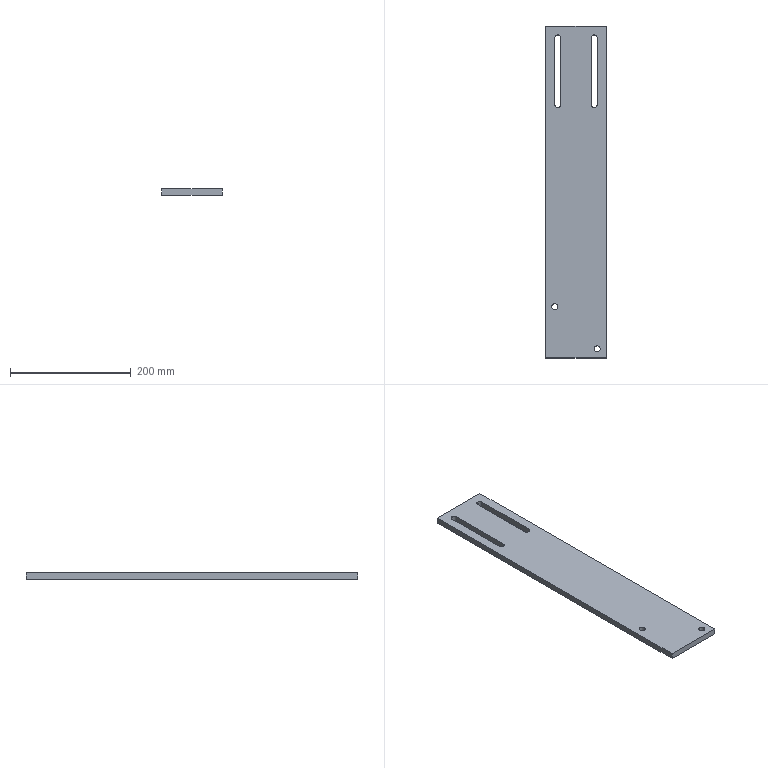Part | SolidWorks | features ICE 2, Extrusion 1 | 1 solid | 26 faces | box 100 x 550 x 10 mm | volume 524777 mm3 | plane 14 | cylinder 12 | commonest cylinder face diameters 9 x8 10 x4
STEP:
#1=CARTESIAN_POINT('',(30.,-260.,0.));
#2=VERTEX_POINT('',#1);
#3=CARTESIAN_POINT('',(40.,-260.,0.));
#4=VERTEX_POINT('',#3);
#5=CARTESIAN_POINT('',(35.,-260.,0.));
#6=DIRECTION('',(0.,0.,1.));
#7=DIRECTION('',(1.,0.,0.));
#8=AXIS2_PLACEMENT_3D('',#5,#6,#7);
#9=CIRCLE('',#8,5.);
#10=EDGE_CURVE('',#2,#4,#9,.T.);
#11=ORIENTED_EDGE('',*,*,#10,.F.);
#12=CARTESIAN_POINT('',(30.,-260.,10.));
#13=VERTEX_POINT('',#12);
#14=CARTESIAN_POINT('',(30.,-260.,0.));
#15=DIRECTION('',(0.,0.,1.));
#16=VECTOR('',#15,1000.);
#17=LINE('',#14,#16);
#18=EDGE_CURVE('',#2,#13,#17,.T.);
#19=ORIENTED_EDGE('',*,*,#18,.T.);
#20=CARTESIAN_POINT('',(40.,-260.,10.));
#21=VERTEX_POINT('',#20);
#22=CARTESIAN_POINT('',(35.,-260.,10.));
#23=DIRECTION('',(0.,0.,1.));
#24=DIRECTION('',(1.,0.,0.));
#25=AXIS2_PLACEMENT_3D('',#22,#23,#24);
#26=CIRCLE('',#25,5.);
#27=EDGE_CURVE('',#13,#21,#26,.T.);
#28=ORIENTED_EDGE('',*,*,#27,.T.);
#29=CARTESIAN_POINT('',(40.,-260.,0.));
#30=DIRECTION('',(0.,0.,1.));
#31=VECTOR('',#30,1000.);
#32=LINE('',#29,#31);
#33=EDGE_CURVE('',#4,#21,#32,.T.);
#34=ORIENTED_EDGE('',*,*,#33,.F.);
#35=EDGE_LOOP('',(#11,#19,#28,#34));
#36=FACE_OUTER_BOUND('',#35,.T.);
#37=CARTESIAN_POINT('',(35.,-260.,0.));
#38=DIRECTION('',(0.,0.,1.));
#39=DIRECTION('',(1.,0.,0.));
#40=AXIS2_PLACEMENT_3D('',#37,#38,#39);
#41=CYLINDRICAL_SURFACE('',#40,5.);
#42=ADVANCED_FACE('',(#36),#41,.F.);
#43=CARTESIAN_POINT('',(-40.,-190.,0.));
#44=VERTEX_POINT('',#43);
#45=CARTESIAN_POINT('',(-30.,-190.,0.));
#46=VERTEX_POINT('',#45);
#47=CARTESIAN_POINT('',(-35.,-190.,0.));
#48=DIRECTION('',(0.,0.,1.));
#49=DIRECTION('',(1.,0.,0.));
#50=AXIS2_PLACEMENT_3D('',#47,#48,#49);
#51=CIRCLE('',#50,5.);
#52=EDGE_CURVE('',#44,#46,#51,.T.);
#53=ORIENTED_EDGE('',*,*,#52,.F.);
#54=CARTESIAN_POINT('',(-40.,-190.,10.));
#55=VERTEX_POINT('',#54);
#56=CARTESIAN_POINT('',(-40.,-190.,0.));
#57=DIRECTION('',(0.,0.,1.));
#58=VECTOR('',#57,1000.);
#59=LINE('',#56,#58);
#60=EDGE_CURVE('',#44,#55,#59,.T.);
#61=ORIENTED_EDGE('',*,*,#60,.T.);
#62=CARTESIAN_POINT('',(-30.,-190.,10.));
#63=VERTEX_POINT('',#62);
#64=CARTESIAN_POINT('',(-35.,-190.,10.));
#65=DIRECTION('',(0.,0.,1.));
#66=DIRECTION('',(1.,0.,0.));
#67=AXIS2_PLACEMENT_3D('',#64,#65,#66);
#68=CIRCLE('',#67,5.);
#69=EDGE_CURVE('',#55,#63,#68,.T.);
#70=ORIENTED_EDGE('',*,*,#69,.T.);
#71=CARTESIAN_POINT('',(-30.,-190.,0.));
#72=DIRECTION('',(0.,0.,1.));
#73=VECTOR('',#72,1000.);
#74=LINE('',#71,#73);
#75=EDGE_CURVE('',#46,#63,#74,.T.);
#76=ORIENTED_EDGE('',*,*,#75,.F.);
#77=EDGE_LOOP('',(#53,#61,#70,#76));
#78=FACE_OUTER_BOUND('',#77,.T.);
#79=CARTESIAN_POINT('',(-35.,-190.,0.));
#80=DIRECTION('',(0.,0.,1.));
#81=DIRECTION('',(1.,0.,0.));
#82=AXIS2_PLACEMENT_3D('',#79,#80,#81);
#83=CYLINDRICAL_SURFACE('',#82,5.);
#84=ADVANCED_FACE('',(#78),#83,.F.);
#85=CARTESIAN_POINT('',(-50.,275.,0.));
#86=VERTEX_POINT('',#85);
#87=CARTESIAN_POINT('',(-50.,-275.,0.));
#88=VERTEX_POINT('',#87);
#89=CARTESIAN_POINT('',(-50.,-275.,0.));
#90=DIRECTION('',(0.,-1.,0.));
#91=VECTOR('',#90,1000.);
#92=LINE('',#89,#91);
#93=EDGE_CURVE('',#86,#88,#92,.T.);
#94=ORIENTED_EDGE('',*,*,#93,.T.);
#95=CARTESIAN_POINT('',(-50.,-275.,10.));
#96=VERTEX_POINT('',#95);
#97=CARTESIAN_POINT('',(-50.,-275.,10.));
#98=DIRECTION('',(0.,0.,-1.));
#99=VECTOR('',#98,1000.);
#100=LINE('',#97,#99);
#101=EDGE_CURVE('',#96,#88,#100,.T.);
#102=ORIENTED_EDGE('',*,*,#101,.F.);
#103=CARTESIAN_POINT('',(-50.,275.,10.));
#104=VERTEX_POINT('',#103);
#105=CARTESIAN_POINT('',(-50.,-275.,10.));
#106=DIRECTION('',(0.,-1.,0.));
#107=VECTOR('',#106,1000.);
#108=LINE('',#105,#107);
#109=EDGE_CURVE('',#104,#96,#108,.T.);
#110=ORIENTED_EDGE('',*,*,#109,.F.);
#111=CARTESIAN_POINT('',(-50.,275.,10.));
#112=DIRECTION('',(0.,0.,-1.));
#113=VECTOR('',#112,1000.);
#114=LINE('',#111,#113);
#115=EDGE_CURVE('',#104,#86,#114,.T.);
#116=ORIENTED_EDGE('',*,*,#115,.T.);
#117=EDGE_LOOP('',(#94,#102,#110,#116));
#118=FACE_OUTER_BOUND('',#117,.T.);
#119=CARTESIAN_POINT('',(-50.,-275.,10.));
#120=DIRECTION('',(1.,0.,0.));
#121=DIRECTION('',(0.,0.,-1.));
#122=AXIS2_PLACEMENT_3D('',#119,#120,#121);
#123=PLANE('',#122);
#124=ADVANCED_FACE('',(#118),#123,.F.);
#125=CARTESIAN_POINT('',(50.,-275.,0.));
#126=VERTEX_POINT('',#125);
#127=CARTESIAN_POINT('',(50.,-275.,0.));
#128=DIRECTION('',(1.,0.,0.));
#129=VECTOR('',#128,1000.);
#130=LINE('',#127,#129);
#131=EDGE_CURVE('',#88,#126,#130,.T.);
#132=ORIENTED_EDGE('',*,*,#131,.T.);
#133=CARTESIAN_POINT('',(50.,-275.,10.));
#134=VERTEX_POINT('',#133);
#135=CARTESIAN_POINT('',(50.,-275.,10.));
#136=DIRECTION('',(0.,0.,-1.));
#137=VECTOR('',#136,1000.);
#138=LINE('',#135,#137);
#139=EDGE_CURVE('',#134,#126,#138,.T.);
#140=ORIENTED_EDGE('',*,*,#139,.F.);
#141=CARTESIAN_POINT('',(50.,-275.,10.));
#142=DIRECTION('',(1.,0.,0.));
#143=VECTOR('',#142,1000.);
#144=LINE('',#141,#143);
#145=EDGE_CURVE('',#96,#134,#144,.T.);
#146=ORIENTED_EDGE('',*,*,#145,.F.);
#147=ORIENTED_EDGE('',*,*,#101,.T.);
#148=EDGE_LOOP('',(#132,#140,#146,#147));
#149=FACE_OUTER_BOUND('',#148,.T.);
#150=CARTESIAN_POINT('',(50.,-275.,10.));
#151=DIRECTION('',(0.,1.,0.));
#152=DIRECTION('',(0.,0.,1.));
#153=AXIS2_PLACEMENT_3D('',#150,#151,#152);
#154=PLANE('',#153);
#155=ADVANCED_FACE('',(#149),#154,.F.);
#156=CARTESIAN_POINT('',(50.,275.,0.));
#157=VERTEX_POINT('',#156);
#158=CARTESIAN_POINT('',(50.,-275.,0.));
#159=DIRECTION('',(0.,1.,0.));
#160=VECTOR('',#159,1000.);
#161=LINE('',#158,#160);
#162=EDGE_CURVE('',#126,#157,#161,.T.);
#163=ORIENTED_EDGE('',*,*,#162,.T.);
#164=CARTESIAN_POINT('',(50.,275.,10.));
#165=VERTEX_POINT('',#164);
#166=CARTESIAN_POINT('',(50.,275.,10.));
#167=DIRECTION('',(0.,0.,-1.));
#168=VECTOR('',#167,1000.);
#169=LINE('',#166,#168);
#170=EDGE_CURVE('',#165,#157,#169,.T.);
#171=ORIENTED_EDGE('',*,*,#170,.F.);
#172=CARTESIAN_POINT('',(50.,-275.,10.));
#173=DIRECTION('',(0.,1.,0.));
#174=VECTOR('',#173,1000.);
#175=LINE('',#172,#174);
#176=EDGE_CURVE('',#134,#165,#175,.T.);
#177=ORIENTED_EDGE('',*,*,#176,.F.);
#178=ORIENTED_EDGE('',*,*,#139,.T.);
#179=EDGE_LOOP('',(#163,#171,#177,#178));
#180=FACE_OUTER_BOUND('',#179,.T.);
#181=CARTESIAN_POINT('',(50.,-275.,10.));
#182=DIRECTION('',(-1.,0.,0.));
#183=DIRECTION('',(0.,0.,1.));
#184=AXIS2_PLACEMENT_3D('',#181,#182,#183);
#185=PLANE('',#184);
#186=ADVANCED_FACE('',(#180),#185,.F.);
#187=CARTESIAN_POINT('',(50.,275.,0.));
#188=DIRECTION('',(-1.,0.,0.));
#189=VECTOR('',#188,1000.);
#190=LINE('',#187,#189);
#191=EDGE_CURVE('',#157,#86,#190,.T.);
#192=ORIENTED_EDGE('',*,*,#191,.T.);
#193=ORIENTED_EDGE('',*,*,#115,.F.);
#194=CARTESIAN_POINT('',(50.,275.,10.));
#195=DIRECTION('',(-1.,0.,0.));
#196=VECTOR('',#195,1000.);
#197=LINE('',#194,#196);
#198=EDGE_CURVE('',#165,#104,#197,.T.);
#199=ORIENTED_EDGE('',*,*,#198,.F.);
#200=ORIENTED_EDGE('',*,*,#170,.T.);
#201=EDGE_LOOP('',(#192,#193,#199,#200));
#202=FACE_OUTER_BOUND('',#201,.T.);
#203=CARTESIAN_POINT('',(50.,275.,10.));
#204=DIRECTION('',(0.,-1.,0.));
#205=DIRECTION('',(0.,0.,-1.));
#206=AXIS2_PLACEMENT_3D('',#203,#204,#205);
#207=PLANE('',#206);
#208=ADVANCED_FACE('',(#202),#207,.F.);
#209=CARTESIAN_POINT('',(-35.,144.6,10.));
#210=VERTEX_POINT('',#209);
#211=CARTESIAN_POINT('',(-30.5,140.1,10.));
#212=VERTEX_POINT('',#211);
#213=CARTESIAN_POINT('',(-30.5,144.6,10.));
#214=DIRECTION('',(0.,0.,1.));
#215=DIRECTION('',(-1.,0.,0.));
#216=AXIS2_PLACEMENT_3D('',#213,#214,#215);
#217=CIRCLE('',#216,4.5);
#218=EDGE_CURVE('',#210,#212,#217,.T.);
#219=ORIENTED_EDGE('',*,*,#218,.F.);
#220=CARTESIAN_POINT('',(-35.,255.6,10.));
#221=VERTEX_POINT('',#220);
#222=CARTESIAN_POINT('',(-35.,144.6,10.));
#223=DIRECTION('',(0.,-1.,0.));
#224=VECTOR('',#223,1000.);
#225=LINE('',#222,#224);
#226=EDGE_CURVE('',#221,#210,#225,.T.);
#227=ORIENTED_EDGE('',*,*,#226,.F.);
#228=CARTESIAN_POINT('',(-30.5,260.1,10.));
#229=VERTEX_POINT('',#228);
#230=CARTESIAN_POINT('',(-30.5,255.6,10.));
#231=DIRECTION('',(0.,0.,1.));
#232=DIRECTION('',(1.,0.,0.));
#233=AXIS2_PLACEMENT_3D('',#230,#231,#232);
#234=CIRCLE('',#233,4.5);
#235=EDGE_CURVE('',#229,#221,#234,.T.);
#236=ORIENTED_EDGE('',*,*,#235,.F.);
#237=CARTESIAN_POINT('',(-29.5,260.1,10.));
#238=VERTEX_POINT('',#237);
#239=CARTESIAN_POINT('',(-29.5,260.1,10.));
#240=DIRECTION('',(-1.,0.,0.));
#241=VECTOR('',#240,1000.);
#242=LINE('',#239,#241);
#243=EDGE_CURVE('',#238,#229,#242,.T.);
#244=ORIENTED_EDGE('',*,*,#243,.F.);
#245=CARTESIAN_POINT('',(-25.,255.6,10.));
#246=VERTEX_POINT('',#245);
#247=CARTESIAN_POINT('',(-29.5,255.6,10.));
#248=DIRECTION('',(0.,0.,1.));
#249=DIRECTION('',(1.,0.,0.));
#250=AXIS2_PLACEMENT_3D('',#247,#248,#249);
#251=CIRCLE('',#250,4.5);
#252=EDGE_CURVE('',#246,#238,#251,.T.);
#253=ORIENTED_EDGE('',*,*,#252,.F.);
#254=CARTESIAN_POINT('',(-25.,144.6,10.));
#255=VERTEX_POINT('',#254);
#256=CARTESIAN_POINT('',(-25.,144.6,10.));
#257=DIRECTION('',(0.,1.,0.));
#258=VECTOR('',#257,1000.);
#259=LINE('',#256,#258);
#260=EDGE_CURVE('',#255,#246,#259,.T.);
#261=ORIENTED_EDGE('',*,*,#260,.F.);
#262=CARTESIAN_POINT('',(-29.5,140.1,10.));
#263=VERTEX_POINT('',#262);
#264=CARTESIAN_POINT('',(-29.5,144.6,10.));
#265=DIRECTION('',(0.,0.,1.));
#266=DIRECTION('',(1.,0.,0.));
#267=AXIS2_PLACEMENT_3D('',#264,#265,#266);
#268=CIRCLE('',#267,4.5);
#269=EDGE_CURVE('',#263,#255,#268,.T.);
#270=ORIENTED_EDGE('',*,*,#269,.F.);
#271=CARTESIAN_POINT('',(-29.5,140.1,10.));
#272=DIRECTION('',(1.,0.,0.));
#273=VECTOR('',#272,1000.);
#274=LINE('',#271,#273);
#275=EDGE_CURVE('',#212,#263,#274,.T.);
#276=ORIENTED_EDGE('',*,*,#275,.F.);
#277=EDGE_LOOP('',(#219,#227,#236,#244,#253,#261,#270,#276));
#278=FACE_BOUND('',#277,.T.);
#279=CARTESIAN_POINT('',(29.5,260.1,10.));
#280=VERTEX_POINT('',#279);
#281=CARTESIAN_POINT('',(25.,255.6,10.));
#282=VERTEX_POINT('',#281);
#283=CARTESIAN_POINT('',(29.5,255.6,10.));
#284=DIRECTION('',(0.,0.,1.));
#285=DIRECTION('',(1.,0.,0.));
#286=AXIS2_PLACEMENT_3D('',#283,#284,#285);
#287=CIRCLE('',#286,4.5);
#288=EDGE_CURVE('',#280,#282,#287,.T.);
#289=ORIENTED_EDGE('',*,*,#288,.F.);
#290=CARTESIAN_POINT('',(30.5,260.1,10.));
#291=VERTEX_POINT('',#290);
#292=CARTESIAN_POINT('',(30.5,260.1,10.));
#293=DIRECTION('',(-1.,0.,0.));
#294=VECTOR('',#293,1000.);
#295=LINE('',#292,#294);
#296=EDGE_CURVE('',#291,#280,#295,.T.);
#297=ORIENTED_EDGE('',*,*,#296,.F.);
#298=CARTESIAN_POINT('',(35.,255.6,10.));
#299=VERTEX_POINT('',#298);
#300=CARTESIAN_POINT('',(30.5,255.6,10.));
#301=DIRECTION('',(0.,0.,1.));
#302=DIRECTION('',(1.,0.,0.));
#303=AXIS2_PLACEMENT_3D('',#300,#301,#302);
#304=CIRCLE('',#303,4.5);
#305=EDGE_CURVE('',#299,#291,#304,.T.);
#306=ORIENTED_EDGE('',*,*,#305,.F.);
#307=CARTESIAN_POINT('',(35.,144.6,10.));
#308=VERTEX_POINT('',#307);
#309=CARTESIAN_POINT('',(35.,144.6,10.));
#310=DIRECTION('',(0.,1.,0.));
#311=VECTOR('',#310,1000.);
#312=LINE('',#309,#311);
#313=EDGE_CURVE('',#308,#299,#312,.T.);
#314=ORIENTED_EDGE('',*,*,#313,.F.);
#315=CARTESIAN_POINT('',(30.5,140.1,10.));
#316=VERTEX_POINT('',#315);
#317=CARTESIAN_POINT('',(30.5,144.6,10.));
#318=DIRECTION('',(0.,0.,1.));
#319=DIRECTION('',(1.,0.,0.));
#320=AXIS2_PLACEMENT_3D('',#317,#318,#319);
#321=CIRCLE('',#320,4.5);
#322=EDGE_CURVE('',#316,#308,#321,.T.);
#323=ORIENTED_EDGE('',*,*,#322,.F.);
#324=CARTESIAN_POINT('',(29.5,140.1,10.));
#325=VERTEX_POINT('',#324);
#326=CARTESIAN_POINT('',(30.5,140.1,10.));
#327=DIRECTION('',(1.,0.,0.));
#328=VECTOR('',#327,1000.);
#329=LINE('',#326,#328);
#330=EDGE_CURVE('',#325,#316,#329,.T.);
#331=ORIENTED_EDGE('',*,*,#330,.F.);
#332=CARTESIAN_POINT('',(25.,144.6,10.));
#333=VERTEX_POINT('',#332);
#334=CARTESIAN_POINT('',(29.5,144.6,10.));
#335=DIRECTION('',(0.,0.,1.));
#336=DIRECTION('',(-1.,0.,0.));
#337=AXIS2_PLACEMENT_3D('',#334,#335,#336);
#338=CIRCLE('',#337,4.5);
#339=EDGE_CURVE('',#333,#325,#338,.T.);
#340=ORIENTED_EDGE('',*,*,#339,.F.);
#341=CARTESIAN_POINT('',(25.,144.6,10.));
#342=DIRECTION('',(0.,-1.,0.));
#343=VECTOR('',#342,1000.);
#344=LINE('',#341,#343);
#345=EDGE_CURVE('',#282,#333,#344,.T.);
#346=ORIENTED_EDGE('',*,*,#345,.F.);
#347=EDGE_LOOP('',(#289,#297,#306,#314,#323,#331,#340,#346));
#348=FACE_BOUND('',#347,.T.);
#349=CARTESIAN_POINT('',(35.,-260.,10.));
#350=DIRECTION('',(0.,0.,1.));
#351=DIRECTION('',(1.,0.,0.));
#352=AXIS2_PLACEMENT_3D('',#349,#350,#351);
#353=CIRCLE('',#352,5.);
#354=EDGE_CURVE('',#21,#13,#353,.T.);
#355=ORIENTED_EDGE('',*,*,#354,.F.);
#356=ORIENTED_EDGE('',*,*,#27,.F.);
#357=EDGE_LOOP('',(#355,#356));
#358=FACE_BOUND('',#357,.T.);
#359=CARTESIAN_POINT('',(-35.,-190.,10.));
#360=DIRECTION('',(0.,0.,1.));
#361=DIRECTION('',(1.,0.,0.));
#362=AXIS2_PLACEMENT_3D('',#359,#360,#361);
#363=CIRCLE('',#362,5.);
#364=EDGE_CURVE('',#63,#55,#363,.T.);
#365=ORIENTED_EDGE('',*,*,#364,.F.);
#366=ORIENTED_EDGE('',*,*,#69,.F.);
#367=EDGE_LOOP('',(#365,#366));
#368=FACE_BOUND('',#367,.T.);
#369=ORIENTED_EDGE('',*,*,#109,.T.);
#370=ORIENTED_EDGE('',*,*,#145,.T.);
#371=ORIENTED_EDGE('',*,*,#176,.T.);
#372=ORIENTED_EDGE('',*,*,#198,.T.);
#373=EDGE_LOOP('',(#369,#370,#371,#372));
#374=FACE_OUTER_BOUND('',#373,.T.);
#375=CARTESIAN_POINT('',(-50.,275.,10.));
#376=DIRECTION('',(0.,0.,1.));
#377=DIRECTION('',(1.,0.,0.));
#378=AXIS2_PLACEMENT_3D('',#375,#376,#377);
#379=PLANE('',#378);
#380=ADVANCED_FACE('',(#278,#348,#358,#368,#374),#379,.T.);
#381=CARTESIAN_POINT('',(-35.,255.6,0.));
#382=VERTEX_POINT('',#381);
#383=CARTESIAN_POINT('',(-35.,144.6,0.));
#384=VERTEX_POINT('',#383);
#385=CARTESIAN_POINT('',(-35.,144.6,0.));
#386=DIRECTION('',(0.,-1.,0.));
#387=VECTOR('',#386,1000.);
#388=LINE('',#385,#387);
#389=EDGE_CURVE('',#382,#384,#388,.T.);
#390=ORIENTED_EDGE('',*,*,#389,.T.);
#391=CARTESIAN_POINT('',(-30.5,140.1,0.));
#392=VERTEX_POINT('',#391);
#393=CARTESIAN_POINT('',(-30.5,144.6,0.));
#394=DIRECTION('',(0.,0.,1.));
#395=DIRECTION('',(-1.,0.,0.));
#396=AXIS2_PLACEMENT_3D('',#393,#394,#395);
#397=CIRCLE('',#396,4.5);
#398=EDGE_CURVE('',#384,#392,#397,.T.);
#399=ORIENTED_EDGE('',*,*,#398,.T.);
#400=CARTESIAN_POINT('',(-29.5,140.1,0.));
#401=VERTEX_POINT('',#400);
#402=CARTESIAN_POINT('',(-29.5,140.1,0.));
#403=DIRECTION('',(1.,0.,0.));
#404=VECTOR('',#403,1000.);
#405=LINE('',#402,#404);
#406=EDGE_CURVE('',#392,#401,#405,.T.);
#407=ORIENTED_EDGE('',*,*,#406,.T.);
#408=CARTESIAN_POINT('',(-25.,144.6,0.));
#409=VERTEX_POINT('',#408);
#410=CARTESIAN_POINT('',(-29.5,144.6,0.));
#411=DIRECTION('',(0.,0.,1.));
#412=DIRECTION('',(1.,0.,0.));
#413=AXIS2_PLACEMENT_3D('',#410,#411,#412);
#414=CIRCLE('',#413,4.5);
#415=EDGE_CURVE('',#401,#409,#414,.T.);
#416=ORIENTED_EDGE('',*,*,#415,.T.);
#417=CARTESIAN_POINT('',(-25.,255.6,0.));
#418=VERTEX_POINT('',#417);
#419=CARTESIAN_POINT('',(-25.,144.6,0.));
#420=DIRECTION('',(0.,1.,0.));
#421=VECTOR('',#420,1000.);
#422=LINE('',#419,#421);
#423=EDGE_CURVE('',#409,#418,#422,.T.);
#424=ORIENTED_EDGE('',*,*,#423,.T.);
#425=CARTESIAN_POINT('',(-29.5,260.1,0.));
#426=VERTEX_POINT('',#425);
#427=CARTESIAN_POINT('',(-29.5,255.6,0.));
#428=DIRECTION('',(0.,0.,1.));
#429=DIRECTION('',(1.,0.,0.));
#430=AXIS2_PLACEMENT_3D('',#427,#428,#429);
#431=CIRCLE('',#430,4.5);
#432=EDGE_CURVE('',#418,#426,#431,.T.);
#433=ORIENTED_EDGE('',*,*,#432,.T.);
#434=CARTESIAN_POINT('',(-30.5,260.1,0.));
#435=VERTEX_POINT('',#434);
#436=CARTESIAN_POINT('',(-29.5,260.1,0.));
#437=DIRECTION('',(-1.,0.,0.));
#438=VECTOR('',#437,1000.);
#439=LINE('',#436,#438);
#440=EDGE_CURVE('',#426,#435,#439,.T.);
#441=ORIENTED_EDGE('',*,*,#440,.T.);
#442=CARTESIAN_POINT('',(-30.5,255.6,0.));
#443=DIRECTION('',(0.,0.,1.));
#444=DIRECTION('',(1.,0.,0.));
#445=AXIS2_PLACEMENT_3D('',#442,#443,#444);
#446=CIRCLE('',#445,4.5);
#447=EDGE_CURVE('',#435,#382,#446,.T.);
#448=ORIENTED_EDGE('',*,*,#447,.T.);
#449=EDGE_LOOP('',(#390,#399,#407,#416,#424,#433,#441,#448));
#450=FACE_BOUND('',#449,.T.);
#451=CARTESIAN_POINT('',(30.5,260.1,0.));
#452=VERTEX_POINT('',#451);
#453=CARTESIAN_POINT('',(29.5,260.1,0.));
#454=VERTEX_POINT('',#453);
#455=CARTESIAN_POINT('',(30.5,260.1,0.));
#456=DIRECTION('',(-1.,0.,0.));
#457=VECTOR('',#456,1000.);
#458=LINE('',#455,#457);
#459=EDGE_CURVE('',#452,#454,#458,.T.);
#460=ORIENTED_EDGE('',*,*,#459,.T.);
#461=CARTESIAN_POINT('',(25.,255.6,0.));
#462=VERTEX_POINT('',#461);
#463=CARTESIAN_POINT('',(29.5,255.6,0.));
#464=DIRECTION('',(0.,0.,1.));
#465=DIRECTION('',(1.,0.,0.));
#466=AXIS2_PLACEMENT_3D('',#463,#464,#465);
#467=CIRCLE('',#466,4.5);
#468=EDGE_CURVE('',#454,#462,#467,.T.);
#469=ORIENTED_EDGE('',*,*,#468,.T.);
#470=CARTESIAN_POINT('',(25.,144.6,0.));
#471=VERTEX_POINT('',#470);
#472=CARTESIAN_POINT('',(25.,144.6,0.));
#473=DIRECTION('',(0.,-1.,0.));
#474=VECTOR('',#473,1000.);
#475=LINE('',#472,#474);
#476=EDGE_CURVE('',#462,#471,#475,.T.);
#477=ORIENTED_EDGE('',*,*,#476,.T.);
#478=CARTESIAN_POINT('',(29.5,140.1,0.));
#479=VERTEX_POINT('',#478);
#480=CARTESIAN_POINT('',(29.5,144.6,0.));
#481=DIRECTION('',(0.,0.,1.));
#482=DIRECTION('',(-1.,0.,0.));
#483=AXIS2_PLACEMENT_3D('',#480,#481,#482);
#484=CIRCLE('',#483,4.5);
#485=EDGE_CURVE('',#471,#479,#484,.T.);
#486=ORIENTED_EDGE('',*,*,#485,.T.);
#487=CARTESIAN_POINT('',(30.5,140.1,0.));
#488=VERTEX_POINT('',#487);
#489=CARTESIAN_POINT('',(30.5,140.1,0.));
#490=DIRECTION('',(1.,0.,0.));
#491=VECTOR('',#490,1000.);
#492=LINE('',#489,#491);
#493=EDGE_CURVE('',#479,#488,#492,.T.);
#494=ORIENTED_EDGE('',*,*,#493,.T.);
#495=CARTESIAN_POINT('',(35.,144.6,0.));
#496=VERTEX_POINT('',#495);
#497=CARTESIAN_POINT('',(30.5,144.6,0.));
#498=DIRECTION('',(0.,0.,1.));
#499=DIRECTION('',(1.,0.,0.));
#500=AXIS2_PLACEMENT_3D('',#497,#498,#499);
#501=CIRCLE('',#500,4.5);
#502=EDGE_CURVE('',#488,#496,#501,.T.);
#503=ORIENTED_EDGE('',*,*,#502,.T.);
#504=CARTESIAN_POINT('',(35.,255.6,0.));
#505=VERTEX_POINT('',#504);
#506=CARTESIAN_POINT('',(35.,144.6,0.));
#507=DIRECTION('',(0.,1.,0.));
#508=VECTOR('',#507,1000.);
#509=LINE('',#506,#508);
#510=EDGE_CURVE('',#496,#505,#509,.T.);
#511=ORIENTED_EDGE('',*,*,#510,.T.);
#512=CARTESIAN_POINT('',(30.5,255.6,0.));
#513=DIRECTION('',(0.,0.,1.));
#514=DIRECTION('',(1.,0.,0.));
#515=AXIS2_PLACEMENT_3D('',#512,#513,#514);
#516=CIRCLE('',#515,4.5);
#517=EDGE_CURVE('',#505,#452,#516,.T.);
#518=ORIENTED_EDGE('',*,*,#517,.T.);
#519=EDGE_LOOP('',(#460,#469,#477,#486,#494,#503,#511,#518));
#520=FACE_BOUND('',#519,.T.);
#521=CARTESIAN_POINT('',(35.,-260.,0.));
#522=DIRECTION('',(0.,0.,1.));
#523=DIRECTION('',(1.,0.,0.));
#524=AXIS2_PLACEMENT_3D('',#521,#522,#523);
#525=CIRCLE('',#524,5.);
#526=EDGE_CURVE('',#4,#2,#525,.T.);
#527=ORIENTED_EDGE('',*,*,#526,.T.);
#528=ORIENTED_EDGE('',*,*,#10,.T.);
#529=EDGE_LOOP('',(#527,#528));
#530=FACE_BOUND('',#529,.T.);
#531=CARTESIAN_POINT('',(-35.,-190.,0.));
#532=DIRECTION('',(0.,0.,1.));
#533=DIRECTION('',(1.,0.,0.));
#534=AXIS2_PLACEMENT_3D('',#531,#532,#533);
#535=CIRCLE('',#534,5.);
#536=EDGE_CURVE('',#46,#44,#535,.T.);
#537=ORIENTED_EDGE('',*,*,#536,.T.);
#538=ORIENTED_EDGE('',*,*,#52,.T.);
#539=EDGE_LOOP('',(#537,#538));
#540=FACE_BOUND('',#539,.T.);
#541=ORIENTED_EDGE('',*,*,#93,.F.);
#542=ORIENTED_EDGE('',*,*,#191,.F.);
#543=ORIENTED_EDGE('',*,*,#162,.F.);
#544=ORIENTED_EDGE('',*,*,#131,.F.);
#545=EDGE_LOOP('',(#541,#542,#543,#544));
#546=FACE_OUTER_BOUND('',#545,.T.);
#547=CARTESIAN_POINT('',(-50.,275.,0.));
#548=DIRECTION('',(0.,0.,1.));
#549=DIRECTION('',(1.,0.,0.));
#550=AXIS2_PLACEMENT_3D('',#547,#548,#549);
#551=PLANE('',#550);
#552=ADVANCED_FACE('',(#450,#520,#530,#540,#546),#551,.F.);
#553=ORIENTED_EDGE('',*,*,#60,.F.);
#554=ORIENTED_EDGE('',*,*,#536,.F.);
#555=ORIENTED_EDGE('',*,*,#75,.T.);
#556=ORIENTED_EDGE('',*,*,#364,.T.);
#557=EDGE_LOOP('',(#553,#554,#555,#556));
#558=FACE_OUTER_BOUND('',#557,.T.);
#559=CARTESIAN_POINT('',(-35.,-190.,0.));
#560=DIRECTION('',(0.,0.,1.));
#561=DIRECTION('',(1.,0.,0.));
#562=AXIS2_PLACEMENT_3D('',#559,#560,#561);
#563=CYLINDRICAL_SURFACE('',#562,5.);
#564=ADVANCED_FACE('',(#558),#563,.F.);
#565=ORIENTED_EDGE('',*,*,#18,.F.);
#566=ORIENTED_EDGE('',*,*,#526,.F.);
#567=ORIENTED_EDGE('',*,*,#33,.T.);
#568=ORIENTED_EDGE('',*,*,#354,.T.);
#569=EDGE_LOOP('',(#565,#566,#567,#568));
#570=FACE_OUTER_BOUND('',#569,.T.);
#571=CARTESIAN_POINT('',(35.,-260.,0.));
#572=DIRECTION('',(0.,0.,1.));
#573=DIRECTION('',(1.,0.,0.));
#574=AXIS2_PLACEMENT_3D('',#571,#572,#573);
#575=CYLINDRICAL_SURFACE('',#574,5.);
#576=ADVANCED_FACE('',(#570),#575,.F.);
#577=ORIENTED_EDGE('',*,*,#288,.T.);
#578=CARTESIAN_POINT('',(25.,255.6,0.));
#579=DIRECTION('',(0.,0.,1.));
#580=VECTOR('',#579,1000.);
#581=LINE('',#578,#580);
#582=EDGE_CURVE('',#462,#282,#581,.T.);
#583=ORIENTED_EDGE('',*,*,#582,.F.);
#584=ORIENTED_EDGE('',*,*,#468,.F.);
#585=CARTESIAN_POINT('',(29.5,260.1,0.));
#586=DIRECTION('',(0.,0.,1.));
#587=VECTOR('',#586,1000.);
#588=LINE('',#585,#587);
#589=EDGE_CURVE('',#454,#280,#588,.T.);
#590=ORIENTED_EDGE('',*,*,#589,.T.);
#591=EDGE_LOOP('',(#577,#583,#584,#590));
#592=FACE_OUTER_BOUND('',#591,.T.);
#593=CARTESIAN_POINT('',(29.5,255.6,0.));
#594=DIRECTION('',(0.,0.,1.));
#595=DIRECTION('',(1.,0.,0.));
#596=AXIS2_PLACEMENT_3D('',#593,#594,#595);
#597=CYLINDRICAL_SURFACE('',#596,4.5);
#598=ADVANCED_FACE('',(#592),#597,.F.);
#599=ORIENTED_EDGE('',*,*,#296,.T.);
#600=ORIENTED_EDGE('',*,*,#589,.F.);
#601=ORIENTED_EDGE('',*,*,#459,.F.);
#602=CARTESIAN_POINT('',(30.5,260.1,0.));
#603=DIRECTION('',(0.,0.,1.));
#604=VECTOR('',#603,1000.);
#605=LINE('',#602,#604);
#606=EDGE_CURVE('',#452,#291,#605,.T.);
#607=ORIENTED_EDGE('',*,*,#606,.T.);
#608=EDGE_LOOP('',(#599,#600,#601,#607));
#609=FACE_OUTER_BOUND('',#608,.T.);
#610=CARTESIAN_POINT('',(30.5,260.1,0.));
#611=DIRECTION('',(0.,1.,0.));
#612=DIRECTION('',(0.,0.,1.));
#613=AXIS2_PLACEMENT_3D('',#610,#611,#612);
#614=PLANE('',#613);
#615=ADVANCED_FACE('',(#609),#614,.F.);
#616=ORIENTED_EDGE('',*,*,#305,.T.);
#617=ORIENTED_EDGE('',*,*,#606,.F.);
#618=ORIENTED_EDGE('',*,*,#517,.F.);
#619=CARTESIAN_POINT('',(35.,255.6,0.));
#620=DIRECTION('',(0.,0.,1.));
#621=VECTOR('',#620,1000.);
#622=LINE('',#619,#621);
#623=EDGE_CURVE('',#505,#299,#622,.T.);
#624=ORIENTED_EDGE('',*,*,#623,.T.);
#625=EDGE_LOOP('',(#616,#617,#618,#624));
#626=FACE_OUTER_BOUND('',#625,.T.);
#627=CARTESIAN_POINT('',(30.5,255.6,0.));
#628=DIRECTION('',(0.,0.,1.));
#629=DIRECTION('',(1.,0.,0.));
#630=AXIS2_PLACEMENT_3D('',#627,#628,#629);
#631=CYLINDRICAL_SURFACE('',#630,4.5);
#632=ADVANCED_FACE('',(#626),#631,.F.);
#633=ORIENTED_EDGE('',*,*,#313,.T.);
#634=ORIENTED_EDGE('',*,*,#623,.F.);
#635=ORIENTED_EDGE('',*,*,#510,.F.);
#636=CARTESIAN_POINT('',(35.,144.6,0.));
#637=DIRECTION('',(0.,0.,1.));
#638=VECTOR('',#637,1000.);
#639=LINE('',#636,#638);
#640=EDGE_CURVE('',#496,#308,#639,.T.);
#641=ORIENTED_EDGE('',*,*,#640,.T.);
#642=EDGE_LOOP('',(#633,#634,#635,#641));
#643=FACE_OUTER_BOUND('',#642,.T.);
#644=CARTESIAN_POINT('',(35.,144.6,0.));
#645=DIRECTION('',(1.,0.,0.));
#646=DIRECTION('',(0.,0.,-1.));
#647=AXIS2_PLACEMENT_3D('',#644,#645,#646);
#648=PLANE('',#647);
#649=ADVANCED_FACE('',(#643),#648,.F.);
#650=ORIENTED_EDGE('',*,*,#322,.T.);
#651=ORIENTED_EDGE('',*,*,#640,.F.);
#652=ORIENTED_EDGE('',*,*,#502,.F.);
#653=CARTESIAN_POINT('',(30.5,140.1,0.));
#654=DIRECTION('',(0.,0.,1.));
#655=VECTOR('',#654,1000.);
#656=LINE('',#653,#655);
#657=EDGE_CURVE('',#488,#316,#656,.T.);
#658=ORIENTED_EDGE('',*,*,#657,.T.);
#659=EDGE_LOOP('',(#650,#651,#652,#658));
#660=FACE_OUTER_BOUND('',#659,.T.);
#661=CARTESIAN_POINT('',(30.5,144.6,0.));
#662=DIRECTION('',(0.,0.,1.));
#663=DIRECTION('',(1.,0.,0.));
#664=AXIS2_PLACEMENT_3D('',#661,#662,#663);
#665=CYLINDRICAL_SURFACE('',#664,4.5);
#666=ADVANCED_FACE('',(#660),#665,.F.);
#667=ORIENTED_EDGE('',*,*,#330,.T.);
#668=ORIENTED_EDGE('',*,*,#657,.F.);
#669=ORIENTED_EDGE('',*,*,#493,.F.);
#670=CARTESIAN_POINT('',(29.5,140.1,0.));
#671=DIRECTION('',(0.,0.,1.));
#672=VECTOR('',#671,1000.);
#673=LINE('',#670,#672);
#674=EDGE_CURVE('',#479,#325,#673,.T.);
#675=ORIENTED_EDGE('',*,*,#674,.T.);
#676=EDGE_LOOP('',(#667,#668,#669,#675));
#677=FACE_OUTER_BOUND('',#676,.T.);
#678=CARTESIAN_POINT('',(30.5,140.1,0.));
#679=DIRECTION('',(0.,-1.,0.));
#680=DIRECTION('',(0.,0.,-1.));
#681=AXIS2_PLACEMENT_3D('',#678,#679,#680);
#682=PLANE('',#681);
#683=ADVANCED_FACE('',(#677),#682,.F.);
#684=ORIENTED_EDGE('',*,*,#339,.T.);
#685=ORIENTED_EDGE('',*,*,#674,.F.);
#686=ORIENTED_EDGE('',*,*,#485,.F.);
#687=CARTESIAN_POINT('',(25.,144.6,0.));
#688=DIRECTION('',(0.,0.,1.));
#689=VECTOR('',#688,1000.);
#690=LINE('',#687,#689);
#691=EDGE_CURVE('',#471,#333,#690,.T.);
#692=ORIENTED_EDGE('',*,*,#691,.T.);
#693=EDGE_LOOP('',(#684,#685,#686,#692));
#694=FACE_OUTER_BOUND('',#693,.T.);
#695=CARTESIAN_POINT('',(29.5,144.6,0.));
#696=DIRECTION('',(0.,0.,1.));
#697=DIRECTION('',(1.,0.,0.));
#698=AXIS2_PLACEMENT_3D('',#695,#696,#697);
#699=CYLINDRICAL_SURFACE('',#698,4.5);
#700=ADVANCED_FACE('',(#694),#699,.F.);
#701=ORIENTED_EDGE('',*,*,#345,.T.);
#702=ORIENTED_EDGE('',*,*,#691,.F.);
#703=ORIENTED_EDGE('',*,*,#476,.F.);
#704=ORIENTED_EDGE('',*,*,#582,.T.);
#705=EDGE_LOOP('',(#701,#702,#703,#704));
#706=FACE_OUTER_BOUND('',#705,.T.);
#707=CARTESIAN_POINT('',(25.,144.6,0.));
#708=DIRECTION('',(-1.,0.,0.));
#709=DIRECTION('',(0.,-1.,0.));
#710=AXIS2_PLACEMENT_3D('',#707,#708,#709);
#711=PLANE('',#710);
#712=ADVANCED_FACE('',(#706),#711,.F.);
#713=ORIENTED_EDGE('',*,*,#218,.T.);
#714=CARTESIAN_POINT('',(-30.5,140.1,0.));
#715=DIRECTION('',(0.,0.,1.));
#716=VECTOR('',#715,1000.);
#717=LINE('',#714,#716);
#718=EDGE_CURVE('',#392,#212,#717,.T.);
#719=ORIENTED_EDGE('',*,*,#718,.F.);
#720=ORIENTED_EDGE('',*,*,#398,.F.);
#721=CARTESIAN_POINT('',(-35.,144.6,0.));
#722=DIRECTION('',(0.,0.,1.));
#723=VECTOR('',#722,1000.);
#724=LINE('',#721,#723);
#725=EDGE_CURVE('',#384,#210,#724,.T.);
#726=ORIENTED_EDGE('',*,*,#725,.T.);
#727=EDGE_LOOP('',(#713,#719,#720,#726));
#728=FACE_OUTER_BOUND('',#727,.T.);
#729=CARTESIAN_POINT('',(-30.5,144.6,0.));
#730=DIRECTION('',(0.,0.,1.));
#731=DIRECTION('',(1.,0.,0.));
#732=AXIS2_PLACEMENT_3D('',#729,#730,#731);
#733=CYLINDRICAL_SURFACE('',#732,4.5);
#734=ADVANCED_FACE('',(#728),#733,.F.);
#735=ORIENTED_EDGE('',*,*,#226,.T.);
#736=ORIENTED_EDGE('',*,*,#725,.F.);
#737=ORIENTED_EDGE('',*,*,#389,.F.);
#738=CARTESIAN_POINT('',(-35.,255.6,0.));
#739=DIRECTION('',(0.,0.,1.));
#740=VECTOR('',#739,1000.);
#741=LINE('',#738,#740);
#742=EDGE_CURVE('',#382,#221,#741,.T.);
#743=ORIENTED_EDGE('',*,*,#742,.T.);
#744=EDGE_LOOP('',(#735,#736,#737,#743));
#745=FACE_OUTER_BOUND('',#744,.T.);
#746=CARTESIAN_POINT('',(-35.,144.6,0.));
#747=DIRECTION('',(-1.,0.,0.));
#748=DIRECTION('',(0.,0.,1.));
#749=AXIS2_PLACEMENT_3D('',#746,#747,#748);
#750=PLANE('',#749);
#751=ADVANCED_FACE('',(#745),#750,.F.);
#752=ORIENTED_EDGE('',*,*,#235,.T.);
#753=ORIENTED_EDGE('',*,*,#742,.F.);
#754=ORIENTED_EDGE('',*,*,#447,.F.);
#755=CARTESIAN_POINT('',(-30.5,260.1,0.));
#756=DIRECTION('',(0.,0.,1.));
#757=VECTOR('',#756,1000.);
#758=LINE('',#755,#757);
#759=EDGE_CURVE('',#435,#229,#758,.T.);
#760=ORIENTED_EDGE('',*,*,#759,.T.);
#761=EDGE_LOOP('',(#752,#753,#754,#760));
#762=FACE_OUTER_BOUND('',#761,.T.);
#763=CARTESIAN_POINT('',(-30.5,255.6,0.));
#764=DIRECTION('',(0.,0.,1.));
#765=DIRECTION('',(1.,0.,0.));
#766=AXIS2_PLACEMENT_3D('',#763,#764,#765);
#767=CYLINDRICAL_SURFACE('',#766,4.5);
#768=ADVANCED_FACE('',(#762),#767,.F.);
#769=ORIENTED_EDGE('',*,*,#243,.T.);
#770=ORIENTED_EDGE('',*,*,#759,.F.);
#771=ORIENTED_EDGE('',*,*,#440,.F.);
#772=CARTESIAN_POINT('',(-29.5,260.1,0.));
#773=DIRECTION('',(0.,0.,1.));
#774=VECTOR('',#773,1000.);
#775=LINE('',#772,#774);
#776=EDGE_CURVE('',#426,#238,#775,.T.);
#777=ORIENTED_EDGE('',*,*,#776,.T.);
#778=EDGE_LOOP('',(#769,#770,#771,#777));
#779=FACE_OUTER_BOUND('',#778,.T.);
#780=CARTESIAN_POINT('',(-29.5,260.1,0.));
#781=DIRECTION('',(0.,1.,0.));
#782=DIRECTION('',(0.,0.,1.));
#783=AXIS2_PLACEMENT_3D('',#780,#781,#782);
#784=PLANE('',#783);
#785=ADVANCED_FACE('',(#779),#784,.F.);
#786=ORIENTED_EDGE('',*,*,#252,.T.);
#787=ORIENTED_EDGE('',*,*,#776,.F.);
#788=ORIENTED_EDGE('',*,*,#432,.F.);
#789=CARTESIAN_POINT('',(-25.,255.6,0.));
#790=DIRECTION('',(0.,0.,1.));
#791=VECTOR('',#790,1000.);
#792=LINE('',#789,#791);
#793=EDGE_CURVE('',#418,#246,#792,.T.);
#794=ORIENTED_EDGE('',*,*,#793,.T.);
#795=EDGE_LOOP('',(#786,#787,#788,#794));
#796=FACE_OUTER_BOUND('',#795,.T.);
#797=CARTESIAN_POINT('',(-29.5,255.6,0.));
#798=DIRECTION('',(0.,0.,1.));
#799=DIRECTION('',(1.,0.,0.));
#800=AXIS2_PLACEMENT_3D('',#797,#798,#799);
#801=CYLINDRICAL_SURFACE('',#800,4.5);
#802=ADVANCED_FACE('',(#796),#801,.F.);
#803=ORIENTED_EDGE('',*,*,#260,.T.);
#804=ORIENTED_EDGE('',*,*,#793,.F.);
#805=ORIENTED_EDGE('',*,*,#423,.F.);
#806=CARTESIAN_POINT('',(-25.,144.6,0.));
#807=DIRECTION('',(0.,0.,1.));
#808=VECTOR('',#807,1000.);
#809=LINE('',#806,#808);
#810=EDGE_CURVE('',#409,#255,#809,.T.);
#811=ORIENTED_EDGE('',*,*,#810,.T.);
#812=EDGE_LOOP('',(#803,#804,#805,#811));
#813=FACE_OUTER_BOUND('',#812,.T.);
#814=CARTESIAN_POINT('',(-25.,144.6,0.));
#815=DIRECTION('',(1.,0.,0.));
#816=DIRECTION('',(0.,0.,-1.));
#817=AXIS2_PLACEMENT_3D('',#814,#815,#816);
#818=PLANE('',#817);
#819=ADVANCED_FACE('',(#813),#818,.F.);
#820=ORIENTED_EDGE('',*,*,#269,.T.);
#821=ORIENTED_EDGE('',*,*,#810,.F.);
#822=ORIENTED_EDGE('',*,*,#415,.F.);
#823=CARTESIAN_POINT('',(-29.5,140.1,0.));
#824=DIRECTION('',(0.,0.,1.));
#825=VECTOR('',#824,1000.);
#826=LINE('',#823,#825);
#827=EDGE_CURVE('',#401,#263,#826,.T.);
#828=ORIENTED_EDGE('',*,*,#827,.T.);
#829=EDGE_LOOP('',(#820,#821,#822,#828));
#830=FACE_OUTER_BOUND('',#829,.T.);
#831=CARTESIAN_POINT('',(-29.5,144.6,0.));
#832=DIRECTION('',(0.,0.,1.));
#833=DIRECTION('',(1.,0.,0.));
#834=AXIS2_PLACEMENT_3D('',#831,#832,#833);
#835=CYLINDRICAL_SURFACE('',#834,4.5);
#836=ADVANCED_FACE('',(#830),#835,.F.);
#837=ORIENTED_EDGE('',*,*,#275,.T.);
#838=ORIENTED_EDGE('',*,*,#827,.F.);
#839=ORIENTED_EDGE('',*,*,#406,.F.);
#840=ORIENTED_EDGE('',*,*,#718,.T.);
#841=EDGE_LOOP('',(#837,#838,#839,#840));
#842=FACE_OUTER_BOUND('',#841,.T.);
#843=CARTESIAN_POINT('',(-29.5,140.1,0.));
#844=DIRECTION('',(0.,-1.,0.));
#845=DIRECTION('',(0.,0.,-1.));
#846=AXIS2_PLACEMENT_3D('',#843,#844,#845);
#847=PLANE('',#846);
#848=ADVANCED_FACE('',(#842),#847,.F.);
#849=CLOSED_SHELL('',(#42,#84,#124,#155,#186,#208,#380,#552,#564,#576,#598,#615,#632,#649,#666,#683,#700,#712,#734,#751,#768,#785,#802,#819,#836,#848));
#850=MANIFOLD_SOLID_BREP('',#849);
#851=CARTESIAN_POINT('',(0.,0.,0.));
#852=DIRECTION('',(0.,0.,1.));
#853=DIRECTION('',(1.,0.,0.));
#854=AXIS2_PLACEMENT_3D('',#851,#852,#853);
#855=(LENGTH_UNIT()NAMED_UNIT(*)SI_UNIT(.MILLI.,.METRE.));
#856=UNCERTAINTY_MEASURE_WITH_UNIT(LENGTH_MEASURE(0.00001),#855,'','');
#857=(NAMED_UNIT(*)PLANE_ANGLE_UNIT()SI_UNIT($,.RADIAN.));
#858=(NAMED_UNIT(*)SI_UNIT($,.STERADIAN.)SOLID_ANGLE_UNIT());
#859=(GEOMETRIC_REPRESENTATION_CONTEXT(3)GLOBAL_UNCERTAINTY_ASSIGNED_CONTEXT((#856))GLOBAL_UNIT_ASSIGNED_CONTEXT((#855,#857,#858))REPRESENTATION_CONTEXT('',''));
#860=ADVANCED_BREP_SHAPE_REPRESENTATION('',(#850,#854),#859);